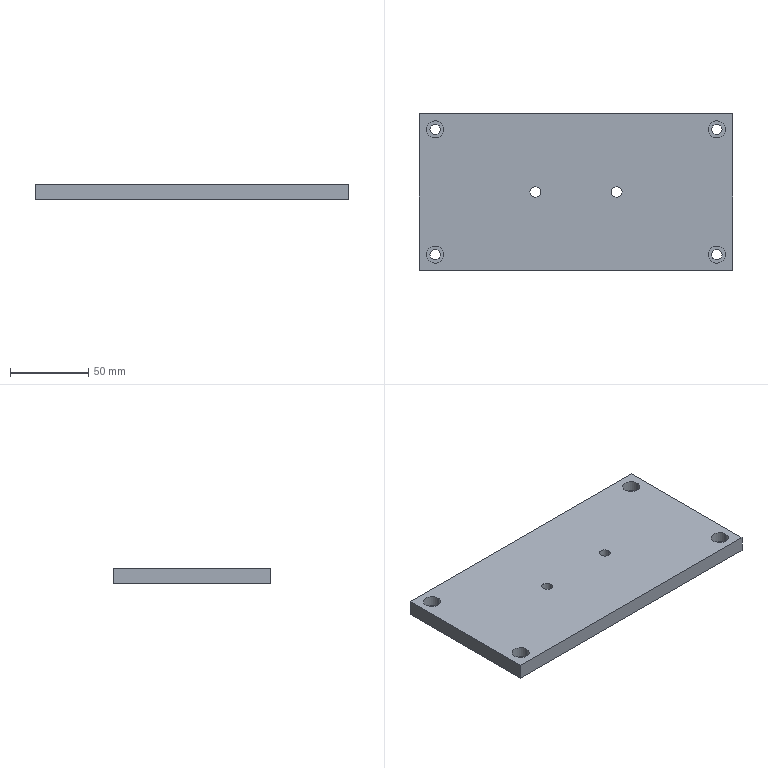Part | STEP file | MYT-A01-P29 | 1 solid | 30 faces | box 200 x 100 x 10 mm | volume 196251 mm3 | cylinder 20 | plane 10 | commonest cylinder face diameters 6.6 x8 11 x8 6.8 x4
STEP:
#1=CARTESIAN_POINT('',(-95.5,40.,3.2));
#2=VERTEX_POINT('',#1);
#3=CARTESIAN_POINT('',(-84.5,40.,3.2));
#4=VERTEX_POINT('',#3);
#5=CARTESIAN_POINT('',(-90.,40.,3.2));
#6=DIRECTION('',(0.,0.,1.));
#7=DIRECTION('',(1.,0.,0.));
#8=AXIS2_PLACEMENT_3D('',#5,#6,#7);
#9=CIRCLE('',#8,5.5);
#10=EDGE_CURVE('',#2,#4,#9,.T.);
#11=ORIENTED_EDGE('',*,*,#10,.F.);
#12=CARTESIAN_POINT('',(-95.5,40.,10.));
#13=VERTEX_POINT('',#12);
#14=CARTESIAN_POINT('',(-95.5,40.,10.));
#15=DIRECTION('',(0.,0.,1.));
#16=VECTOR('',#15,1000.);
#17=LINE('',#14,#16);
#18=EDGE_CURVE('',#2,#13,#17,.T.);
#19=ORIENTED_EDGE('',*,*,#18,.T.);
#20=CARTESIAN_POINT('',(-84.5,40.,10.));
#21=VERTEX_POINT('',#20);
#22=CARTESIAN_POINT('',(-90.,40.,10.));
#23=DIRECTION('',(0.,0.,1.));
#24=DIRECTION('',(1.,0.,0.));
#25=AXIS2_PLACEMENT_3D('',#22,#23,#24);
#26=CIRCLE('',#25,5.5);
#27=EDGE_CURVE('',#13,#21,#26,.T.);
#28=ORIENTED_EDGE('',*,*,#27,.T.);
#29=CARTESIAN_POINT('',(-84.5,40.,10.));
#30=DIRECTION('',(0.,0.,1.));
#31=VECTOR('',#30,1000.);
#32=LINE('',#29,#31);
#33=EDGE_CURVE('',#4,#21,#32,.T.);
#34=ORIENTED_EDGE('',*,*,#33,.F.);
#35=EDGE_LOOP('',(#11,#19,#28,#34));
#36=FACE_OUTER_BOUND('',#35,.T.);
#37=CARTESIAN_POINT('',(-90.,40.,10.));
#38=DIRECTION('',(0.,0.,1.));
#39=DIRECTION('',(1.,0.,0.));
#40=AXIS2_PLACEMENT_3D('',#37,#38,#39);
#41=CYLINDRICAL_SURFACE('',#40,5.5);
#42=ADVANCED_FACE('',(#36),#41,.F.);
#43=CARTESIAN_POINT('',(-93.3,40.,0.));
#44=VERTEX_POINT('',#43);
#45=CARTESIAN_POINT('',(-86.7,40.,0.));
#46=VERTEX_POINT('',#45);
#47=CARTESIAN_POINT('',(-90.,40.,0.));
#48=DIRECTION('',(0.,0.,1.));
#49=DIRECTION('',(1.,0.,0.));
#50=AXIS2_PLACEMENT_3D('',#47,#48,#49);
#51=CIRCLE('',#50,3.3);
#52=EDGE_CURVE('',#44,#46,#51,.T.);
#53=ORIENTED_EDGE('',*,*,#52,.F.);
#54=CARTESIAN_POINT('',(-93.3,40.,3.2));
#55=VERTEX_POINT('',#54);
#56=CARTESIAN_POINT('',(-93.3,40.,10.));
#57=DIRECTION('',(0.,0.,1.));
#58=VECTOR('',#57,1000.);
#59=LINE('',#56,#58);
#60=EDGE_CURVE('',#44,#55,#59,.T.);
#61=ORIENTED_EDGE('',*,*,#60,.T.);
#62=CARTESIAN_POINT('',(-86.7,40.,3.2));
#63=VERTEX_POINT('',#62);
#64=CARTESIAN_POINT('',(-90.,40.,3.2));
#65=DIRECTION('',(0.,0.,1.));
#66=DIRECTION('',(1.,0.,0.));
#67=AXIS2_PLACEMENT_3D('',#64,#65,#66);
#68=CIRCLE('',#67,3.3);
#69=EDGE_CURVE('',#55,#63,#68,.T.);
#70=ORIENTED_EDGE('',*,*,#69,.T.);
#71=CARTESIAN_POINT('',(-86.7,40.,10.));
#72=DIRECTION('',(0.,0.,1.));
#73=VECTOR('',#72,1000.);
#74=LINE('',#71,#73);
#75=EDGE_CURVE('',#46,#63,#74,.T.);
#76=ORIENTED_EDGE('',*,*,#75,.F.);
#77=EDGE_LOOP('',(#53,#61,#70,#76));
#78=FACE_OUTER_BOUND('',#77,.T.);
#79=CARTESIAN_POINT('',(-90.,40.,10.));
#80=DIRECTION('',(0.,0.,1.));
#81=DIRECTION('',(1.,0.,0.));
#82=AXIS2_PLACEMENT_3D('',#79,#80,#81);
#83=CYLINDRICAL_SURFACE('',#82,3.3);
#84=ADVANCED_FACE('',(#78),#83,.F.);
#85=CARTESIAN_POINT('',(84.5,40.,3.2));
#86=VERTEX_POINT('',#85);
#87=CARTESIAN_POINT('',(95.5,40.,3.2));
#88=VERTEX_POINT('',#87);
#89=CARTESIAN_POINT('',(90.,40.,3.2));
#90=DIRECTION('',(0.,0.,1.));
#91=DIRECTION('',(1.,0.,0.));
#92=AXIS2_PLACEMENT_3D('',#89,#90,#91);
#93=CIRCLE('',#92,5.5);
#94=EDGE_CURVE('',#86,#88,#93,.T.);
#95=ORIENTED_EDGE('',*,*,#94,.F.);
#96=CARTESIAN_POINT('',(84.5,40.,10.));
#97=VERTEX_POINT('',#96);
#98=CARTESIAN_POINT('',(84.5,40.,10.));
#99=DIRECTION('',(0.,0.,1.));
#100=VECTOR('',#99,1000.);
#101=LINE('',#98,#100);
#102=EDGE_CURVE('',#86,#97,#101,.T.);
#103=ORIENTED_EDGE('',*,*,#102,.T.);
#104=CARTESIAN_POINT('',(95.5,40.,10.));
#105=VERTEX_POINT('',#104);
#106=CARTESIAN_POINT('',(90.,40.,10.));
#107=DIRECTION('',(0.,0.,1.));
#108=DIRECTION('',(1.,0.,0.));
#109=AXIS2_PLACEMENT_3D('',#106,#107,#108);
#110=CIRCLE('',#109,5.5);
#111=EDGE_CURVE('',#97,#105,#110,.T.);
#112=ORIENTED_EDGE('',*,*,#111,.T.);
#113=CARTESIAN_POINT('',(95.5,40.,10.));
#114=DIRECTION('',(0.,0.,1.));
#115=VECTOR('',#114,1000.);
#116=LINE('',#113,#115);
#117=EDGE_CURVE('',#88,#105,#116,.T.);
#118=ORIENTED_EDGE('',*,*,#117,.F.);
#119=EDGE_LOOP('',(#95,#103,#112,#118));
#120=FACE_OUTER_BOUND('',#119,.T.);
#121=CARTESIAN_POINT('',(90.,40.,10.));
#122=DIRECTION('',(0.,0.,1.));
#123=DIRECTION('',(1.,0.,0.));
#124=AXIS2_PLACEMENT_3D('',#121,#122,#123);
#125=CYLINDRICAL_SURFACE('',#124,5.5);
#126=ADVANCED_FACE('',(#120),#125,.F.);
#127=CARTESIAN_POINT('',(86.7,40.,0.));
#128=VERTEX_POINT('',#127);
#129=CARTESIAN_POINT('',(93.3,40.,0.));
#130=VERTEX_POINT('',#129);
#131=CARTESIAN_POINT('',(90.,40.,0.));
#132=DIRECTION('',(0.,0.,1.));
#133=DIRECTION('',(1.,0.,0.));
#134=AXIS2_PLACEMENT_3D('',#131,#132,#133);
#135=CIRCLE('',#134,3.3);
#136=EDGE_CURVE('',#128,#130,#135,.T.);
#137=ORIENTED_EDGE('',*,*,#136,.F.);
#138=CARTESIAN_POINT('',(86.7,40.,3.2));
#139=VERTEX_POINT('',#138);
#140=CARTESIAN_POINT('',(86.7,40.,10.));
#141=DIRECTION('',(0.,0.,1.));
#142=VECTOR('',#141,1000.);
#143=LINE('',#140,#142);
#144=EDGE_CURVE('',#128,#139,#143,.T.);
#145=ORIENTED_EDGE('',*,*,#144,.T.);
#146=CARTESIAN_POINT('',(93.3,40.,3.2));
#147=VERTEX_POINT('',#146);
#148=CARTESIAN_POINT('',(90.,40.,3.2));
#149=DIRECTION('',(0.,0.,1.));
#150=DIRECTION('',(1.,0.,0.));
#151=AXIS2_PLACEMENT_3D('',#148,#149,#150);
#152=CIRCLE('',#151,3.3);
#153=EDGE_CURVE('',#139,#147,#152,.T.);
#154=ORIENTED_EDGE('',*,*,#153,.T.);
#155=CARTESIAN_POINT('',(93.3,40.,10.));
#156=DIRECTION('',(0.,0.,1.));
#157=VECTOR('',#156,1000.);
#158=LINE('',#155,#157);
#159=EDGE_CURVE('',#130,#147,#158,.T.);
#160=ORIENTED_EDGE('',*,*,#159,.F.);
#161=EDGE_LOOP('',(#137,#145,#154,#160));
#162=FACE_OUTER_BOUND('',#161,.T.);
#163=CARTESIAN_POINT('',(90.,40.,10.));
#164=DIRECTION('',(0.,0.,1.));
#165=DIRECTION('',(1.,0.,0.));
#166=AXIS2_PLACEMENT_3D('',#163,#164,#165);
#167=CYLINDRICAL_SURFACE('',#166,3.3);
#168=ADVANCED_FACE('',(#162),#167,.F.);
#169=CARTESIAN_POINT('',(84.5,-40.,3.2));
#170=VERTEX_POINT('',#169);
#171=CARTESIAN_POINT('',(95.5,-40.,3.2));
#172=VERTEX_POINT('',#171);
#173=CARTESIAN_POINT('',(90.,-40.,3.2));
#174=DIRECTION('',(0.,0.,1.));
#175=DIRECTION('',(1.,0.,0.));
#176=AXIS2_PLACEMENT_3D('',#173,#174,#175);
#177=CIRCLE('',#176,5.5);
#178=EDGE_CURVE('',#170,#172,#177,.T.);
#179=ORIENTED_EDGE('',*,*,#178,.F.);
#180=CARTESIAN_POINT('',(84.5,-40.,10.));
#181=VERTEX_POINT('',#180);
#182=CARTESIAN_POINT('',(84.5,-40.,10.));
#183=DIRECTION('',(0.,0.,1.));
#184=VECTOR('',#183,1000.);
#185=LINE('',#182,#184);
#186=EDGE_CURVE('',#170,#181,#185,.T.);
#187=ORIENTED_EDGE('',*,*,#186,.T.);
#188=CARTESIAN_POINT('',(95.5,-40.,10.));
#189=VERTEX_POINT('',#188);
#190=CARTESIAN_POINT('',(90.,-40.,10.));
#191=DIRECTION('',(0.,0.,1.));
#192=DIRECTION('',(1.,0.,0.));
#193=AXIS2_PLACEMENT_3D('',#190,#191,#192);
#194=CIRCLE('',#193,5.5);
#195=EDGE_CURVE('',#181,#189,#194,.T.);
#196=ORIENTED_EDGE('',*,*,#195,.T.);
#197=CARTESIAN_POINT('',(95.5,-40.,10.));
#198=DIRECTION('',(0.,0.,1.));
#199=VECTOR('',#198,1000.);
#200=LINE('',#197,#199);
#201=EDGE_CURVE('',#172,#189,#200,.T.);
#202=ORIENTED_EDGE('',*,*,#201,.F.);
#203=EDGE_LOOP('',(#179,#187,#196,#202));
#204=FACE_OUTER_BOUND('',#203,.T.);
#205=CARTESIAN_POINT('',(90.,-40.,10.));
#206=DIRECTION('',(0.,0.,1.));
#207=DIRECTION('',(1.,0.,0.));
#208=AXIS2_PLACEMENT_3D('',#205,#206,#207);
#209=CYLINDRICAL_SURFACE('',#208,5.5);
#210=ADVANCED_FACE('',(#204),#209,.F.);
#211=CARTESIAN_POINT('',(86.7,-40.,0.));
#212=VERTEX_POINT('',#211);
#213=CARTESIAN_POINT('',(93.3,-40.,0.));
#214=VERTEX_POINT('',#213);
#215=CARTESIAN_POINT('',(90.,-40.,0.));
#216=DIRECTION('',(0.,0.,1.));
#217=DIRECTION('',(1.,0.,0.));
#218=AXIS2_PLACEMENT_3D('',#215,#216,#217);
#219=CIRCLE('',#218,3.3);
#220=EDGE_CURVE('',#212,#214,#219,.T.);
#221=ORIENTED_EDGE('',*,*,#220,.F.);
#222=CARTESIAN_POINT('',(86.7,-40.,3.2));
#223=VERTEX_POINT('',#222);
#224=CARTESIAN_POINT('',(86.7,-40.,10.));
#225=DIRECTION('',(0.,0.,1.));
#226=VECTOR('',#225,1000.);
#227=LINE('',#224,#226);
#228=EDGE_CURVE('',#212,#223,#227,.T.);
#229=ORIENTED_EDGE('',*,*,#228,.T.);
#230=CARTESIAN_POINT('',(93.3,-40.,3.2));
#231=VERTEX_POINT('',#230);
#232=CARTESIAN_POINT('',(90.,-40.,3.2));
#233=DIRECTION('',(0.,0.,1.));
#234=DIRECTION('',(1.,0.,0.));
#235=AXIS2_PLACEMENT_3D('',#232,#233,#234);
#236=CIRCLE('',#235,3.3);
#237=EDGE_CURVE('',#223,#231,#236,.T.);
#238=ORIENTED_EDGE('',*,*,#237,.T.);
#239=CARTESIAN_POINT('',(93.3,-40.,10.));
#240=DIRECTION('',(0.,0.,1.));
#241=VECTOR('',#240,1000.);
#242=LINE('',#239,#241);
#243=EDGE_CURVE('',#214,#231,#242,.T.);
#244=ORIENTED_EDGE('',*,*,#243,.F.);
#245=EDGE_LOOP('',(#221,#229,#238,#244));
#246=FACE_OUTER_BOUND('',#245,.T.);
#247=CARTESIAN_POINT('',(90.,-40.,10.));
#248=DIRECTION('',(0.,0.,1.));
#249=DIRECTION('',(1.,0.,0.));
#250=AXIS2_PLACEMENT_3D('',#247,#248,#249);
#251=CYLINDRICAL_SURFACE('',#250,3.3);
#252=ADVANCED_FACE('',(#246),#251,.F.);
#253=CARTESIAN_POINT('',(-95.5,-40.,3.2));
#254=VERTEX_POINT('',#253);
#255=CARTESIAN_POINT('',(-84.5,-40.,3.2));
#256=VERTEX_POINT('',#255);
#257=CARTESIAN_POINT('',(-90.,-40.,3.2));
#258=DIRECTION('',(0.,0.,1.));
#259=DIRECTION('',(1.,0.,0.));
#260=AXIS2_PLACEMENT_3D('',#257,#258,#259);
#261=CIRCLE('',#260,5.5);
#262=EDGE_CURVE('',#254,#256,#261,.T.);
#263=ORIENTED_EDGE('',*,*,#262,.F.);
#264=CARTESIAN_POINT('',(-95.5,-40.,10.));
#265=VERTEX_POINT('',#264);
#266=CARTESIAN_POINT('',(-95.5,-40.,10.));
#267=DIRECTION('',(0.,0.,1.));
#268=VECTOR('',#267,1000.);
#269=LINE('',#266,#268);
#270=EDGE_CURVE('',#254,#265,#269,.T.);
#271=ORIENTED_EDGE('',*,*,#270,.T.);
#272=CARTESIAN_POINT('',(-84.5,-40.,10.));
#273=VERTEX_POINT('',#272);
#274=CARTESIAN_POINT('',(-90.,-40.,10.));
#275=DIRECTION('',(0.,0.,1.));
#276=DIRECTION('',(1.,0.,0.));
#277=AXIS2_PLACEMENT_3D('',#274,#275,#276);
#278=CIRCLE('',#277,5.5);
#279=EDGE_CURVE('',#265,#273,#278,.T.);
#280=ORIENTED_EDGE('',*,*,#279,.T.);
#281=CARTESIAN_POINT('',(-84.5,-40.,10.));
#282=DIRECTION('',(0.,0.,1.));
#283=VECTOR('',#282,1000.);
#284=LINE('',#281,#283);
#285=EDGE_CURVE('',#256,#273,#284,.T.);
#286=ORIENTED_EDGE('',*,*,#285,.F.);
#287=EDGE_LOOP('',(#263,#271,#280,#286));
#288=FACE_OUTER_BOUND('',#287,.T.);
#289=CARTESIAN_POINT('',(-90.,-40.,10.));
#290=DIRECTION('',(0.,0.,1.));
#291=DIRECTION('',(1.,0.,0.));
#292=AXIS2_PLACEMENT_3D('',#289,#290,#291);
#293=CYLINDRICAL_SURFACE('',#292,5.5);
#294=ADVANCED_FACE('',(#288),#293,.F.);
#295=CARTESIAN_POINT('',(-93.3,-40.,0.));
#296=VERTEX_POINT('',#295);
#297=CARTESIAN_POINT('',(-86.7,-40.,0.));
#298=VERTEX_POINT('',#297);
#299=CARTESIAN_POINT('',(-90.,-40.,0.));
#300=DIRECTION('',(0.,0.,1.));
#301=DIRECTION('',(1.,0.,0.));
#302=AXIS2_PLACEMENT_3D('',#299,#300,#301);
#303=CIRCLE('',#302,3.3);
#304=EDGE_CURVE('',#296,#298,#303,.T.);
#305=ORIENTED_EDGE('',*,*,#304,.F.);
#306=CARTESIAN_POINT('',(-93.3,-40.,3.2));
#307=VERTEX_POINT('',#306);
#308=CARTESIAN_POINT('',(-93.3,-40.,10.));
#309=DIRECTION('',(0.,0.,1.));
#310=VECTOR('',#309,1000.);
#311=LINE('',#308,#310);
#312=EDGE_CURVE('',#296,#307,#311,.T.);
#313=ORIENTED_EDGE('',*,*,#312,.T.);
#314=CARTESIAN_POINT('',(-86.7,-40.,3.2));
#315=VERTEX_POINT('',#314);
#316=CARTESIAN_POINT('',(-90.,-40.,3.2));
#317=DIRECTION('',(0.,0.,1.));
#318=DIRECTION('',(1.,0.,0.));
#319=AXIS2_PLACEMENT_3D('',#316,#317,#318);
#320=CIRCLE('',#319,3.3);
#321=EDGE_CURVE('',#307,#315,#320,.T.);
#322=ORIENTED_EDGE('',*,*,#321,.T.);
#323=CARTESIAN_POINT('',(-86.7,-40.,10.));
#324=DIRECTION('',(0.,0.,1.));
#325=VECTOR('',#324,1000.);
#326=LINE('',#323,#325);
#327=EDGE_CURVE('',#298,#315,#326,.T.);
#328=ORIENTED_EDGE('',*,*,#327,.F.);
#329=EDGE_LOOP('',(#305,#313,#322,#328));
#330=FACE_OUTER_BOUND('',#329,.T.);
#331=CARTESIAN_POINT('',(-90.,-40.,10.));
#332=DIRECTION('',(0.,0.,1.));
#333=DIRECTION('',(1.,0.,0.));
#334=AXIS2_PLACEMENT_3D('',#331,#332,#333);
#335=CYLINDRICAL_SURFACE('',#334,3.3);
#336=ADVANCED_FACE('',(#330),#335,.F.);
#337=CARTESIAN_POINT('',(-29.4,0.,0.));
#338=VERTEX_POINT('',#337);
#339=CARTESIAN_POINT('',(-22.6,0.,0.));
#340=VERTEX_POINT('',#339);
#341=CARTESIAN_POINT('',(-26.,0.,0.));
#342=DIRECTION('',(0.,0.,1.));
#343=DIRECTION('',(1.,0.,0.));
#344=AXIS2_PLACEMENT_3D('',#341,#342,#343);
#345=CIRCLE('',#344,3.4);
#346=EDGE_CURVE('',#338,#340,#345,.T.);
#347=ORIENTED_EDGE('',*,*,#346,.F.);
#348=CARTESIAN_POINT('',(-29.4,0.,10.));
#349=VERTEX_POINT('',#348);
#350=CARTESIAN_POINT('',(-29.4,0.,10.));
#351=DIRECTION('',(0.,0.,1.));
#352=VECTOR('',#351,1000.);
#353=LINE('',#350,#352);
#354=EDGE_CURVE('',#338,#349,#353,.T.);
#355=ORIENTED_EDGE('',*,*,#354,.T.);
#356=CARTESIAN_POINT('',(-22.6,0.,10.));
#357=VERTEX_POINT('',#356);
#358=CARTESIAN_POINT('',(-26.,0.,10.));
#359=DIRECTION('',(0.,0.,1.));
#360=DIRECTION('',(1.,0.,0.));
#361=AXIS2_PLACEMENT_3D('',#358,#359,#360);
#362=CIRCLE('',#361,3.4);
#363=EDGE_CURVE('',#349,#357,#362,.T.);
#364=ORIENTED_EDGE('',*,*,#363,.T.);
#365=CARTESIAN_POINT('',(-22.6,0.,10.));
#366=DIRECTION('',(0.,0.,1.));
#367=VECTOR('',#366,1000.);
#368=LINE('',#365,#367);
#369=EDGE_CURVE('',#340,#357,#368,.T.);
#370=ORIENTED_EDGE('',*,*,#369,.F.);
#371=EDGE_LOOP('',(#347,#355,#364,#370));
#372=FACE_OUTER_BOUND('',#371,.T.);
#373=CARTESIAN_POINT('',(-26.,0.,10.));
#374=DIRECTION('',(0.,0.,1.));
#375=DIRECTION('',(1.,0.,0.));
#376=AXIS2_PLACEMENT_3D('',#373,#374,#375);
#377=CYLINDRICAL_SURFACE('',#376,3.4);
#378=ADVANCED_FACE('',(#372),#377,.F.);
#379=CARTESIAN_POINT('',(22.6,0.,0.));
#380=VERTEX_POINT('',#379);
#381=CARTESIAN_POINT('',(29.4,0.,0.));
#382=VERTEX_POINT('',#381);
#383=CARTESIAN_POINT('',(26.,0.,0.));
#384=DIRECTION('',(0.,0.,1.));
#385=DIRECTION('',(1.,0.,0.));
#386=AXIS2_PLACEMENT_3D('',#383,#384,#385);
#387=CIRCLE('',#386,3.4);
#388=EDGE_CURVE('',#380,#382,#387,.T.);
#389=ORIENTED_EDGE('',*,*,#388,.F.);
#390=CARTESIAN_POINT('',(22.6,0.,10.));
#391=VERTEX_POINT('',#390);
#392=CARTESIAN_POINT('',(22.6,0.,10.));
#393=DIRECTION('',(0.,0.,1.));
#394=VECTOR('',#393,1000.);
#395=LINE('',#392,#394);
#396=EDGE_CURVE('',#380,#391,#395,.T.);
#397=ORIENTED_EDGE('',*,*,#396,.T.);
#398=CARTESIAN_POINT('',(29.4,0.,10.));
#399=VERTEX_POINT('',#398);
#400=CARTESIAN_POINT('',(26.,0.,10.));
#401=DIRECTION('',(0.,0.,1.));
#402=DIRECTION('',(1.,0.,0.));
#403=AXIS2_PLACEMENT_3D('',#400,#401,#402);
#404=CIRCLE('',#403,3.4);
#405=EDGE_CURVE('',#391,#399,#404,.T.);
#406=ORIENTED_EDGE('',*,*,#405,.T.);
#407=CARTESIAN_POINT('',(29.4,0.,10.));
#408=DIRECTION('',(0.,0.,1.));
#409=VECTOR('',#408,1000.);
#410=LINE('',#407,#409);
#411=EDGE_CURVE('',#382,#399,#410,.T.);
#412=ORIENTED_EDGE('',*,*,#411,.F.);
#413=EDGE_LOOP('',(#389,#397,#406,#412));
#414=FACE_OUTER_BOUND('',#413,.T.);
#415=CARTESIAN_POINT('',(26.,0.,10.));
#416=DIRECTION('',(0.,0.,1.));
#417=DIRECTION('',(1.,0.,0.));
#418=AXIS2_PLACEMENT_3D('',#415,#416,#417);
#419=CYLINDRICAL_SURFACE('',#418,3.4);
#420=ADVANCED_FACE('',(#414),#419,.F.);
#421=CARTESIAN_POINT('',(100.,-50.,0.));
#422=VERTEX_POINT('',#421);
#423=CARTESIAN_POINT('',(100.,50.,0.));
#424=VERTEX_POINT('',#423);
#425=CARTESIAN_POINT('',(100.,50.,0.));
#426=DIRECTION('',(0.,1.,0.));
#427=VECTOR('',#426,1000.);
#428=LINE('',#425,#427);
#429=EDGE_CURVE('',#422,#424,#428,.T.);
#430=ORIENTED_EDGE('',*,*,#429,.T.);
#431=CARTESIAN_POINT('',(100.,50.,10.));
#432=VERTEX_POINT('',#431);
#433=CARTESIAN_POINT('',(100.,50.,10.));
#434=DIRECTION('',(0.,0.,-1.));
#435=VECTOR('',#434,1000.);
#436=LINE('',#433,#435);
#437=EDGE_CURVE('',#432,#424,#436,.T.);
#438=ORIENTED_EDGE('',*,*,#437,.F.);
#439=CARTESIAN_POINT('',(100.,-50.,10.));
#440=VERTEX_POINT('',#439);
#441=CARTESIAN_POINT('',(100.,50.,10.));
#442=DIRECTION('',(0.,1.,0.));
#443=VECTOR('',#442,1000.);
#444=LINE('',#441,#443);
#445=EDGE_CURVE('',#440,#432,#444,.T.);
#446=ORIENTED_EDGE('',*,*,#445,.F.);
#447=CARTESIAN_POINT('',(100.,-50.,10.));
#448=DIRECTION('',(0.,0.,-1.));
#449=VECTOR('',#448,1000.);
#450=LINE('',#447,#449);
#451=EDGE_CURVE('',#440,#422,#450,.T.);
#452=ORIENTED_EDGE('',*,*,#451,.T.);
#453=EDGE_LOOP('',(#430,#438,#446,#452));
#454=FACE_OUTER_BOUND('',#453,.T.);
#455=CARTESIAN_POINT('',(100.,50.,10.));
#456=DIRECTION('',(-1.,0.,0.));
#457=DIRECTION('',(0.,-1.,0.));
#458=AXIS2_PLACEMENT_3D('',#455,#456,#457);
#459=PLANE('',#458);
#460=ADVANCED_FACE('',(#454),#459,.F.);
#461=CARTESIAN_POINT('',(-100.,50.,0.));
#462=VERTEX_POINT('',#461);
#463=CARTESIAN_POINT('',(-100.,50.,0.));
#464=DIRECTION('',(-1.,0.,0.));
#465=VECTOR('',#464,1000.);
#466=LINE('',#463,#465);
#467=EDGE_CURVE('',#424,#462,#466,.T.);
#468=ORIENTED_EDGE('',*,*,#467,.T.);
#469=CARTESIAN_POINT('',(-100.,50.,10.));
#470=VERTEX_POINT('',#469);
#471=CARTESIAN_POINT('',(-100.,50.,10.));
#472=DIRECTION('',(0.,0.,-1.));
#473=VECTOR('',#472,1000.);
#474=LINE('',#471,#473);
#475=EDGE_CURVE('',#470,#462,#474,.T.);
#476=ORIENTED_EDGE('',*,*,#475,.F.);
#477=CARTESIAN_POINT('',(-100.,50.,10.));
#478=DIRECTION('',(-1.,0.,0.));
#479=VECTOR('',#478,1000.);
#480=LINE('',#477,#479);
#481=EDGE_CURVE('',#432,#470,#480,.T.);
#482=ORIENTED_EDGE('',*,*,#481,.F.);
#483=ORIENTED_EDGE('',*,*,#437,.T.);
#484=EDGE_LOOP('',(#468,#476,#482,#483));
#485=FACE_OUTER_BOUND('',#484,.T.);
#486=CARTESIAN_POINT('',(-100.,50.,10.));
#487=DIRECTION('',(0.,-1.,0.));
#488=DIRECTION('',(0.,0.,-1.));
#489=AXIS2_PLACEMENT_3D('',#486,#487,#488);
#490=PLANE('',#489);
#491=ADVANCED_FACE('',(#485),#490,.F.);
#492=CARTESIAN_POINT('',(-100.,-50.,0.));
#493=VERTEX_POINT('',#492);
#494=CARTESIAN_POINT('',(-100.,50.,0.));
#495=DIRECTION('',(0.,-1.,0.));
#496=VECTOR('',#495,1000.);
#497=LINE('',#494,#496);
#498=EDGE_CURVE('',#462,#493,#497,.T.);
#499=ORIENTED_EDGE('',*,*,#498,.T.);
#500=CARTESIAN_POINT('',(-100.,-50.,10.));
#501=VERTEX_POINT('',#500);
#502=CARTESIAN_POINT('',(-100.,-50.,10.));
#503=DIRECTION('',(0.,0.,-1.));
#504=VECTOR('',#503,1000.);
#505=LINE('',#502,#504);
#506=EDGE_CURVE('',#501,#493,#505,.T.);
#507=ORIENTED_EDGE('',*,*,#506,.F.);
#508=CARTESIAN_POINT('',(-100.,50.,10.));
#509=DIRECTION('',(0.,-1.,0.));
#510=VECTOR('',#509,1000.);
#511=LINE('',#508,#510);
#512=EDGE_CURVE('',#470,#501,#511,.T.);
#513=ORIENTED_EDGE('',*,*,#512,.F.);
#514=ORIENTED_EDGE('',*,*,#475,.T.);
#515=EDGE_LOOP('',(#499,#507,#513,#514));
#516=FACE_OUTER_BOUND('',#515,.T.);
#517=CARTESIAN_POINT('',(-100.,50.,10.));
#518=DIRECTION('',(1.,0.,0.));
#519=DIRECTION('',(0.,1.,0.));
#520=AXIS2_PLACEMENT_3D('',#517,#518,#519);
#521=PLANE('',#520);
#522=ADVANCED_FACE('',(#516),#521,.F.);
#523=CARTESIAN_POINT('',(-100.,-50.,0.));
#524=DIRECTION('',(1.,0.,0.));
#525=VECTOR('',#524,1000.);
#526=LINE('',#523,#525);
#527=EDGE_CURVE('',#493,#422,#526,.T.);
#528=ORIENTED_EDGE('',*,*,#527,.T.);
#529=ORIENTED_EDGE('',*,*,#451,.F.);
#530=CARTESIAN_POINT('',(-100.,-50.,10.));
#531=DIRECTION('',(1.,0.,0.));
#532=VECTOR('',#531,1000.);
#533=LINE('',#530,#532);
#534=EDGE_CURVE('',#501,#440,#533,.T.);
#535=ORIENTED_EDGE('',*,*,#534,.F.);
#536=ORIENTED_EDGE('',*,*,#506,.T.);
#537=EDGE_LOOP('',(#528,#529,#535,#536));
#538=FACE_OUTER_BOUND('',#537,.T.);
#539=CARTESIAN_POINT('',(-100.,-50.,10.));
#540=DIRECTION('',(0.,1.,0.));
#541=DIRECTION('',(0.,0.,1.));
#542=AXIS2_PLACEMENT_3D('',#539,#540,#541);
#543=PLANE('',#542);
#544=ADVANCED_FACE('',(#538),#543,.F.);
#545=CARTESIAN_POINT('',(-90.,40.,10.));
#546=DIRECTION('',(0.,0.,1.));
#547=DIRECTION('',(1.,0.,0.));
#548=AXIS2_PLACEMENT_3D('',#545,#546,#547);
#549=CIRCLE('',#548,5.5);
#550=EDGE_CURVE('',#21,#13,#549,.T.);
#551=ORIENTED_EDGE('',*,*,#550,.F.);
#552=ORIENTED_EDGE('',*,*,#27,.F.);
#553=EDGE_LOOP('',(#551,#552));
#554=FACE_BOUND('',#553,.T.);
#555=CARTESIAN_POINT('',(90.,40.,10.));
#556=DIRECTION('',(0.,0.,1.));
#557=DIRECTION('',(1.,0.,0.));
#558=AXIS2_PLACEMENT_3D('',#555,#556,#557);
#559=CIRCLE('',#558,5.5);
#560=EDGE_CURVE('',#105,#97,#559,.T.);
#561=ORIENTED_EDGE('',*,*,#560,.F.);
#562=ORIENTED_EDGE('',*,*,#111,.F.);
#563=EDGE_LOOP('',(#561,#562));
#564=FACE_BOUND('',#563,.T.);
#565=CARTESIAN_POINT('',(90.,-40.,10.));
#566=DIRECTION('',(0.,0.,1.));
#567=DIRECTION('',(1.,0.,0.));
#568=AXIS2_PLACEMENT_3D('',#565,#566,#567);
#569=CIRCLE('',#568,5.5);
#570=EDGE_CURVE('',#189,#181,#569,.T.);
#571=ORIENTED_EDGE('',*,*,#570,.F.);
#572=ORIENTED_EDGE('',*,*,#195,.F.);
#573=EDGE_LOOP('',(#571,#572));
#574=FACE_BOUND('',#573,.T.);
#575=CARTESIAN_POINT('',(-90.,-40.,10.));
#576=DIRECTION('',(0.,0.,1.));
#577=DIRECTION('',(1.,0.,0.));
#578=AXIS2_PLACEMENT_3D('',#575,#576,#577);
#579=CIRCLE('',#578,5.5);
#580=EDGE_CURVE('',#273,#265,#579,.T.);
#581=ORIENTED_EDGE('',*,*,#580,.F.);
#582=ORIENTED_EDGE('',*,*,#279,.F.);
#583=EDGE_LOOP('',(#581,#582));
#584=FACE_BOUND('',#583,.T.);
#585=CARTESIAN_POINT('',(-26.,0.,10.));
#586=DIRECTION('',(0.,0.,1.));
#587=DIRECTION('',(1.,0.,0.));
#588=AXIS2_PLACEMENT_3D('',#585,#586,#587);
#589=CIRCLE('',#588,3.4);
#590=EDGE_CURVE('',#357,#349,#589,.T.);
#591=ORIENTED_EDGE('',*,*,#590,.F.);
#592=ORIENTED_EDGE('',*,*,#363,.F.);
#593=EDGE_LOOP('',(#591,#592));
#594=FACE_BOUND('',#593,.T.);
#595=CARTESIAN_POINT('',(26.,0.,10.));
#596=DIRECTION('',(0.,0.,1.));
#597=DIRECTION('',(1.,0.,0.));
#598=AXIS2_PLACEMENT_3D('',#595,#596,#597);
#599=CIRCLE('',#598,3.4);
#600=EDGE_CURVE('',#399,#391,#599,.T.);
#601=ORIENTED_EDGE('',*,*,#600,.F.);
#602=ORIENTED_EDGE('',*,*,#405,.F.);
#603=EDGE_LOOP('',(#601,#602));
#604=FACE_BOUND('',#603,.T.);
#605=ORIENTED_EDGE('',*,*,#445,.T.);
#606=ORIENTED_EDGE('',*,*,#481,.T.);
#607=ORIENTED_EDGE('',*,*,#512,.T.);
#608=ORIENTED_EDGE('',*,*,#534,.T.);
#609=EDGE_LOOP('',(#605,#606,#607,#608));
#610=FACE_OUTER_BOUND('',#609,.T.);
#611=CARTESIAN_POINT('',(0.,0.,10.));
#612=DIRECTION('',(0.,0.,1.));
#613=DIRECTION('',(1.,0.,0.));
#614=AXIS2_PLACEMENT_3D('',#611,#612,#613);
#615=PLANE('',#614);
#616=ADVANCED_FACE('',(#554,#564,#574,#584,#594,#604,#610),#615,.T.);
#617=CARTESIAN_POINT('',(-90.,40.,0.));
#618=DIRECTION('',(0.,0.,1.));
#619=DIRECTION('',(1.,0.,0.));
#620=AXIS2_PLACEMENT_3D('',#617,#618,#619);
#621=CIRCLE('',#620,3.3);
#622=EDGE_CURVE('',#46,#44,#621,.T.);
#623=ORIENTED_EDGE('',*,*,#622,.T.);
#624=ORIENTED_EDGE('',*,*,#52,.T.);
#625=EDGE_LOOP('',(#623,#624));
#626=FACE_BOUND('',#625,.T.);
#627=CARTESIAN_POINT('',(90.,40.,0.));
#628=DIRECTION('',(0.,0.,1.));
#629=DIRECTION('',(1.,0.,0.));
#630=AXIS2_PLACEMENT_3D('',#627,#628,#629);
#631=CIRCLE('',#630,3.3);
#632=EDGE_CURVE('',#130,#128,#631,.T.);
#633=ORIENTED_EDGE('',*,*,#632,.T.);
#634=ORIENTED_EDGE('',*,*,#136,.T.);
#635=EDGE_LOOP('',(#633,#634));
#636=FACE_BOUND('',#635,.T.);
#637=CARTESIAN_POINT('',(90.,-40.,0.));
#638=DIRECTION('',(0.,0.,1.));
#639=DIRECTION('',(1.,0.,0.));
#640=AXIS2_PLACEMENT_3D('',#637,#638,#639);
#641=CIRCLE('',#640,3.3);
#642=EDGE_CURVE('',#214,#212,#641,.T.);
#643=ORIENTED_EDGE('',*,*,#642,.T.);
#644=ORIENTED_EDGE('',*,*,#220,.T.);
#645=EDGE_LOOP('',(#643,#644));
#646=FACE_BOUND('',#645,.T.);
#647=CARTESIAN_POINT('',(-90.,-40.,0.));
#648=DIRECTION('',(0.,0.,1.));
#649=DIRECTION('',(1.,0.,0.));
#650=AXIS2_PLACEMENT_3D('',#647,#648,#649);
#651=CIRCLE('',#650,3.3);
#652=EDGE_CURVE('',#298,#296,#651,.T.);
#653=ORIENTED_EDGE('',*,*,#652,.T.);
#654=ORIENTED_EDGE('',*,*,#304,.T.);
#655=EDGE_LOOP('',(#653,#654));
#656=FACE_BOUND('',#655,.T.);
#657=CARTESIAN_POINT('',(-26.,0.,0.));
#658=DIRECTION('',(0.,0.,1.));
#659=DIRECTION('',(1.,0.,0.));
#660=AXIS2_PLACEMENT_3D('',#657,#658,#659);
#661=CIRCLE('',#660,3.4);
#662=EDGE_CURVE('',#340,#338,#661,.T.);
#663=ORIENTED_EDGE('',*,*,#662,.T.);
#664=ORIENTED_EDGE('',*,*,#346,.T.);
#665=EDGE_LOOP('',(#663,#664));
#666=FACE_BOUND('',#665,.T.);
#667=CARTESIAN_POINT('',(26.,0.,0.));
#668=DIRECTION('',(0.,0.,1.));
#669=DIRECTION('',(1.,0.,0.));
#670=AXIS2_PLACEMENT_3D('',#667,#668,#669);
#671=CIRCLE('',#670,3.4);
#672=EDGE_CURVE('',#382,#380,#671,.T.);
#673=ORIENTED_EDGE('',*,*,#672,.T.);
#674=ORIENTED_EDGE('',*,*,#388,.T.);
#675=EDGE_LOOP('',(#673,#674));
#676=FACE_BOUND('',#675,.T.);
#677=ORIENTED_EDGE('',*,*,#429,.F.);
#678=ORIENTED_EDGE('',*,*,#527,.F.);
#679=ORIENTED_EDGE('',*,*,#498,.F.);
#680=ORIENTED_EDGE('',*,*,#467,.F.);
#681=EDGE_LOOP('',(#677,#678,#679,#680));
#682=FACE_OUTER_BOUND('',#681,.T.);
#683=CARTESIAN_POINT('',(0.,0.,0.));
#684=DIRECTION('',(0.,0.,1.));
#685=DIRECTION('',(1.,0.,0.));
#686=AXIS2_PLACEMENT_3D('',#683,#684,#685);
#687=PLANE('',#686);
#688=ADVANCED_FACE('',(#626,#636,#646,#656,#666,#676,#682),#687,.F.);
#689=ORIENTED_EDGE('',*,*,#396,.F.);
#690=ORIENTED_EDGE('',*,*,#672,.F.);
#691=ORIENTED_EDGE('',*,*,#411,.T.);
#692=ORIENTED_EDGE('',*,*,#600,.T.);
#693=EDGE_LOOP('',(#689,#690,#691,#692));
#694=FACE_OUTER_BOUND('',#693,.T.);
#695=CARTESIAN_POINT('',(26.,0.,10.));
#696=DIRECTION('',(0.,0.,1.));
#697=DIRECTION('',(1.,0.,0.));
#698=AXIS2_PLACEMENT_3D('',#695,#696,#697);
#699=CYLINDRICAL_SURFACE('',#698,3.4);
#700=ADVANCED_FACE('',(#694),#699,.F.);
#701=ORIENTED_EDGE('',*,*,#354,.F.);
#702=ORIENTED_EDGE('',*,*,#662,.F.);
#703=ORIENTED_EDGE('',*,*,#369,.T.);
#704=ORIENTED_EDGE('',*,*,#590,.T.);
#705=EDGE_LOOP('',(#701,#702,#703,#704));
#706=FACE_OUTER_BOUND('',#705,.T.);
#707=CARTESIAN_POINT('',(-26.,0.,10.));
#708=DIRECTION('',(0.,0.,1.));
#709=DIRECTION('',(1.,0.,0.));
#710=AXIS2_PLACEMENT_3D('',#707,#708,#709);
#711=CYLINDRICAL_SURFACE('',#710,3.4);
#712=ADVANCED_FACE('',(#706),#711,.F.);
#713=ORIENTED_EDGE('',*,*,#312,.F.);
#714=ORIENTED_EDGE('',*,*,#652,.F.);
#715=ORIENTED_EDGE('',*,*,#327,.T.);
#716=CARTESIAN_POINT('',(-90.,-40.,3.2));
#717=DIRECTION('',(0.,0.,1.));
#718=DIRECTION('',(1.,0.,0.));
#719=AXIS2_PLACEMENT_3D('',#716,#717,#718);
#720=CIRCLE('',#719,3.3);
#721=EDGE_CURVE('',#315,#307,#720,.T.);
#722=ORIENTED_EDGE('',*,*,#721,.T.);
#723=EDGE_LOOP('',(#713,#714,#715,#722));
#724=FACE_OUTER_BOUND('',#723,.T.);
#725=CARTESIAN_POINT('',(-90.,-40.,10.));
#726=DIRECTION('',(0.,0.,1.));
#727=DIRECTION('',(1.,0.,0.));
#728=AXIS2_PLACEMENT_3D('',#725,#726,#727);
#729=CYLINDRICAL_SURFACE('',#728,3.3);
#730=ADVANCED_FACE('',(#724),#729,.F.);
#731=ORIENTED_EDGE('',*,*,#721,.F.);
#732=ORIENTED_EDGE('',*,*,#321,.F.);
#733=EDGE_LOOP('',(#731,#732));
#734=FACE_BOUND('',#733,.T.);
#735=CARTESIAN_POINT('',(-90.,-40.,3.2));
#736=DIRECTION('',(0.,0.,1.));
#737=DIRECTION('',(1.,0.,0.));
#738=AXIS2_PLACEMENT_3D('',#735,#736,#737);
#739=CIRCLE('',#738,5.5);
#740=EDGE_CURVE('',#256,#254,#739,.T.);
#741=ORIENTED_EDGE('',*,*,#740,.T.);
#742=ORIENTED_EDGE('',*,*,#262,.T.);
#743=EDGE_LOOP('',(#741,#742));
#744=FACE_OUTER_BOUND('',#743,.T.);
#745=CARTESIAN_POINT('',(-86.7,-40.,3.2));
#746=DIRECTION('',(0.,0.,-1.));
#747=DIRECTION('',(-1.,0.,0.));
#748=AXIS2_PLACEMENT_3D('',#745,#746,#747);
#749=PLANE('',#748);
#750=ADVANCED_FACE('',(#734,#744),#749,.F.);
#751=ORIENTED_EDGE('',*,*,#270,.F.);
#752=ORIENTED_EDGE('',*,*,#740,.F.);
#753=ORIENTED_EDGE('',*,*,#285,.T.);
#754=ORIENTED_EDGE('',*,*,#580,.T.);
#755=EDGE_LOOP('',(#751,#752,#753,#754));
#756=FACE_OUTER_BOUND('',#755,.T.);
#757=CARTESIAN_POINT('',(-90.,-40.,10.));
#758=DIRECTION('',(0.,0.,1.));
#759=DIRECTION('',(1.,0.,0.));
#760=AXIS2_PLACEMENT_3D('',#757,#758,#759);
#761=CYLINDRICAL_SURFACE('',#760,5.5);
#762=ADVANCED_FACE('',(#756),#761,.F.);
#763=ORIENTED_EDGE('',*,*,#228,.F.);
#764=ORIENTED_EDGE('',*,*,#642,.F.);
#765=ORIENTED_EDGE('',*,*,#243,.T.);
#766=CARTESIAN_POINT('',(90.,-40.,3.2));
#767=DIRECTION('',(0.,0.,1.));
#768=DIRECTION('',(1.,0.,0.));
#769=AXIS2_PLACEMENT_3D('',#766,#767,#768);
#770=CIRCLE('',#769,3.3);
#771=EDGE_CURVE('',#231,#223,#770,.T.);
#772=ORIENTED_EDGE('',*,*,#771,.T.);
#773=EDGE_LOOP('',(#763,#764,#765,#772));
#774=FACE_OUTER_BOUND('',#773,.T.);
#775=CARTESIAN_POINT('',(90.,-40.,10.));
#776=DIRECTION('',(0.,0.,1.));
#777=DIRECTION('',(1.,0.,0.));
#778=AXIS2_PLACEMENT_3D('',#775,#776,#777);
#779=CYLINDRICAL_SURFACE('',#778,3.3);
#780=ADVANCED_FACE('',(#774),#779,.F.);
#781=ORIENTED_EDGE('',*,*,#771,.F.);
#782=ORIENTED_EDGE('',*,*,#237,.F.);
#783=EDGE_LOOP('',(#781,#782));
#784=FACE_BOUND('',#783,.T.);
#785=CARTESIAN_POINT('',(90.,-40.,3.2));
#786=DIRECTION('',(0.,0.,1.));
#787=DIRECTION('',(1.,0.,0.));
#788=AXIS2_PLACEMENT_3D('',#785,#786,#787);
#789=CIRCLE('',#788,5.5);
#790=EDGE_CURVE('',#172,#170,#789,.T.);
#791=ORIENTED_EDGE('',*,*,#790,.T.);
#792=ORIENTED_EDGE('',*,*,#178,.T.);
#793=EDGE_LOOP('',(#791,#792));
#794=FACE_OUTER_BOUND('',#793,.T.);
#795=CARTESIAN_POINT('',(93.3,-40.,3.2));
#796=DIRECTION('',(0.,0.,-1.));
#797=DIRECTION('',(-1.,0.,0.));
#798=AXIS2_PLACEMENT_3D('',#795,#796,#797);
#799=PLANE('',#798);
#800=ADVANCED_FACE('',(#784,#794),#799,.F.);
#801=ORIENTED_EDGE('',*,*,#186,.F.);
#802=ORIENTED_EDGE('',*,*,#790,.F.);
#803=ORIENTED_EDGE('',*,*,#201,.T.);
#804=ORIENTED_EDGE('',*,*,#570,.T.);
#805=EDGE_LOOP('',(#801,#802,#803,#804));
#806=FACE_OUTER_BOUND('',#805,.T.);
#807=CARTESIAN_POINT('',(90.,-40.,10.));
#808=DIRECTION('',(0.,0.,1.));
#809=DIRECTION('',(1.,0.,0.));
#810=AXIS2_PLACEMENT_3D('',#807,#808,#809);
#811=CYLINDRICAL_SURFACE('',#810,5.5);
#812=ADVANCED_FACE('',(#806),#811,.F.);
#813=ORIENTED_EDGE('',*,*,#144,.F.);
#814=ORIENTED_EDGE('',*,*,#632,.F.);
#815=ORIENTED_EDGE('',*,*,#159,.T.);
#816=CARTESIAN_POINT('',(90.,40.,3.2));
#817=DIRECTION('',(0.,0.,1.));
#818=DIRECTION('',(1.,0.,0.));
#819=AXIS2_PLACEMENT_3D('',#816,#817,#818);
#820=CIRCLE('',#819,3.3);
#821=EDGE_CURVE('',#147,#139,#820,.T.);
#822=ORIENTED_EDGE('',*,*,#821,.T.);
#823=EDGE_LOOP('',(#813,#814,#815,#822));
#824=FACE_OUTER_BOUND('',#823,.T.);
#825=CARTESIAN_POINT('',(90.,40.,10.));
#826=DIRECTION('',(0.,0.,1.));
#827=DIRECTION('',(1.,0.,0.));
#828=AXIS2_PLACEMENT_3D('',#825,#826,#827);
#829=CYLINDRICAL_SURFACE('',#828,3.3);
#830=ADVANCED_FACE('',(#824),#829,.F.);
#831=ORIENTED_EDGE('',*,*,#821,.F.);
#832=ORIENTED_EDGE('',*,*,#153,.F.);
#833=EDGE_LOOP('',(#831,#832));
#834=FACE_BOUND('',#833,.T.);
#835=CARTESIAN_POINT('',(90.,40.,3.2));
#836=DIRECTION('',(0.,0.,1.));
#837=DIRECTION('',(1.,0.,0.));
#838=AXIS2_PLACEMENT_3D('',#835,#836,#837);
#839=CIRCLE('',#838,5.5);
#840=EDGE_CURVE('',#88,#86,#839,.T.);
#841=ORIENTED_EDGE('',*,*,#840,.T.);
#842=ORIENTED_EDGE('',*,*,#94,.T.);
#843=EDGE_LOOP('',(#841,#842));
#844=FACE_OUTER_BOUND('',#843,.T.);
#845=CARTESIAN_POINT('',(93.3,40.,3.2));
#846=DIRECTION('',(0.,0.,-1.));
#847=DIRECTION('',(-1.,0.,0.));
#848=AXIS2_PLACEMENT_3D('',#845,#846,#847);
#849=PLANE('',#848);
#850=ADVANCED_FACE('',(#834,#844),#849,.F.);
#851=ORIENTED_EDGE('',*,*,#102,.F.);
#852=ORIENTED_EDGE('',*,*,#840,.F.);
#853=ORIENTED_EDGE('',*,*,#117,.T.);
#854=ORIENTED_EDGE('',*,*,#560,.T.);
#855=EDGE_LOOP('',(#851,#852,#853,#854));
#856=FACE_OUTER_BOUND('',#855,.T.);
#857=CARTESIAN_POINT('',(90.,40.,10.));
#858=DIRECTION('',(0.,0.,1.));
#859=DIRECTION('',(1.,0.,0.));
#860=AXIS2_PLACEMENT_3D('',#857,#858,#859);
#861=CYLINDRICAL_SURFACE('',#860,5.5);
#862=ADVANCED_FACE('',(#856),#861,.F.);
#863=ORIENTED_EDGE('',*,*,#60,.F.);
#864=ORIENTED_EDGE('',*,*,#622,.F.);
#865=ORIENTED_EDGE('',*,*,#75,.T.);
#866=CARTESIAN_POINT('',(-90.,40.,3.2));
#867=DIRECTION('',(0.,0.,1.));
#868=DIRECTION('',(1.,0.,0.));
#869=AXIS2_PLACEMENT_3D('',#866,#867,#868);
#870=CIRCLE('',#869,3.3);
#871=EDGE_CURVE('',#63,#55,#870,.T.);
#872=ORIENTED_EDGE('',*,*,#871,.T.);
#873=EDGE_LOOP('',(#863,#864,#865,#872));
#874=FACE_OUTER_BOUND('',#873,.T.);
#875=CARTESIAN_POINT('',(-90.,40.,10.));
#876=DIRECTION('',(0.,0.,1.));
#877=DIRECTION('',(1.,0.,0.));
#878=AXIS2_PLACEMENT_3D('',#875,#876,#877);
#879=CYLINDRICAL_SURFACE('',#878,3.3);
#880=ADVANCED_FACE('',(#874),#879,.F.);
#881=ORIENTED_EDGE('',*,*,#871,.F.);
#882=ORIENTED_EDGE('',*,*,#69,.F.);
#883=EDGE_LOOP('',(#881,#882));
#884=FACE_BOUND('',#883,.T.);
#885=CARTESIAN_POINT('',(-90.,40.,3.2));
#886=DIRECTION('',(0.,0.,1.));
#887=DIRECTION('',(1.,0.,0.));
#888=AXIS2_PLACEMENT_3D('',#885,#886,#887);
#889=CIRCLE('',#888,5.5);
#890=EDGE_CURVE('',#4,#2,#889,.T.);
#891=ORIENTED_EDGE('',*,*,#890,.T.);
#892=ORIENTED_EDGE('',*,*,#10,.T.);
#893=EDGE_LOOP('',(#891,#892));
#894=FACE_OUTER_BOUND('',#893,.T.);
#895=CARTESIAN_POINT('',(-86.7,40.,3.2));
#896=DIRECTION('',(0.,0.,-1.));
#897=DIRECTION('',(-1.,0.,0.));
#898=AXIS2_PLACEMENT_3D('',#895,#896,#897);
#899=PLANE('',#898);
#900=ADVANCED_FACE('',(#884,#894),#899,.F.);
#901=ORIENTED_EDGE('',*,*,#18,.F.);
#902=ORIENTED_EDGE('',*,*,#890,.F.);
#903=ORIENTED_EDGE('',*,*,#33,.T.);
#904=ORIENTED_EDGE('',*,*,#550,.T.);
#905=EDGE_LOOP('',(#901,#902,#903,#904));
#906=FACE_OUTER_BOUND('',#905,.T.);
#907=CARTESIAN_POINT('',(-90.,40.,10.));
#908=DIRECTION('',(0.,0.,1.));
#909=DIRECTION('',(1.,0.,0.));
#910=AXIS2_PLACEMENT_3D('',#907,#908,#909);
#911=CYLINDRICAL_SURFACE('',#910,5.5);
#912=ADVANCED_FACE('',(#906),#911,.F.);
#913=CLOSED_SHELL('',(#42,#84,#126,#168,#210,#252,#294,#336,#378,#420,#460,#491,#522,#544,#616,#688,#700,#712,#730,#750,#762,#780,#800,#812,#830,#850,#862,#880,#900,#912));
#914=MANIFOLD_SOLID_BREP('',#913);
#915=CARTESIAN_POINT('',(0.,0.,0.));
#916=DIRECTION('',(0.,0.,1.));
#917=DIRECTION('',(1.,0.,0.));
#918=AXIS2_PLACEMENT_3D('',#915,#916,#917);
#919=(LENGTH_UNIT()NAMED_UNIT(*)SI_UNIT(.MILLI.,.METRE.));
#920=UNCERTAINTY_MEASURE_WITH_UNIT(LENGTH_MEASURE(0.00001),#919,'','');
#921=(NAMED_UNIT(*)PLANE_ANGLE_UNIT()SI_UNIT($,.RADIAN.));
#922=(NAMED_UNIT(*)SI_UNIT($,.STERADIAN.)SOLID_ANGLE_UNIT());
#923=(GEOMETRIC_REPRESENTATION_CONTEXT(3)GLOBAL_UNCERTAINTY_ASSIGNED_CONTEXT((#920))GLOBAL_UNIT_ASSIGNED_CONTEXT((#919,#921,#922))REPRESENTATION_CONTEXT('',''));
#924=ADVANCED_BREP_SHAPE_REPRESENTATION('',(#914,#918),#923);